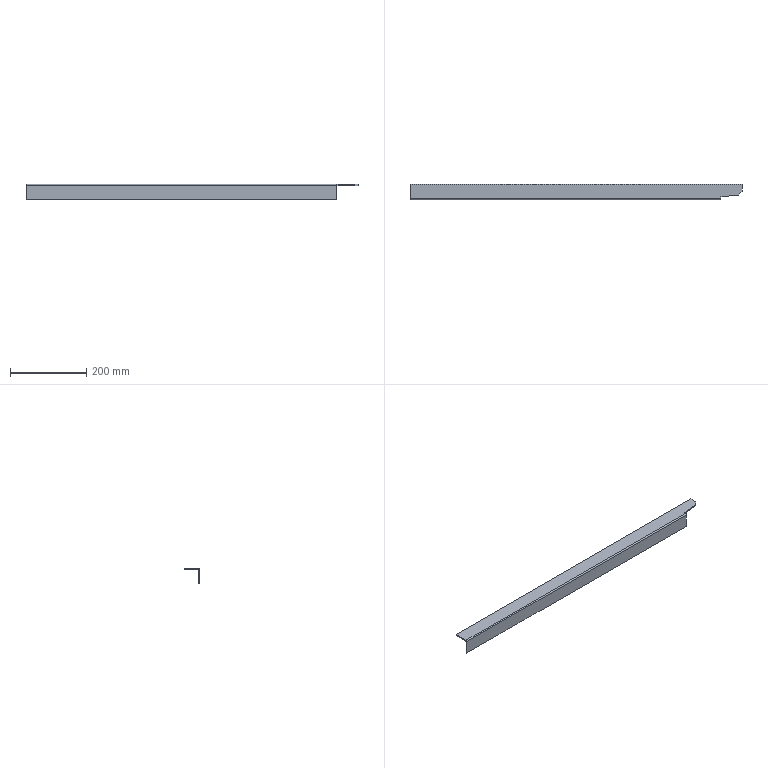Part | SolidWorks | 1 solid | 18 faces | box 873.5 x 40 x 40 mm | volume 192005 mm3 | plane 16 | cylinder 2 | commonest cylinder face diameters 0.2 x1 6.2 x1
STEP:
#1=CARTESIAN_POINT('',(380.25,0.,-40.));
#2=VERTEX_POINT('',#1);
#3=CARTESIAN_POINT('',(380.25,0.,-3.1));
#4=VERTEX_POINT('',#3);
#5=CARTESIAN_POINT('',(380.25,0.,0.));
#6=DIRECTION('',(0.,0.,1.));
#7=VECTOR('',#6,1000.);
#8=LINE('',#5,#7);
#9=EDGE_CURVE('',#2,#4,#8,.T.);
#10=ORIENTED_EDGE('',*,*,#9,.T.);
#11=CARTESIAN_POINT('',(-436.75,0.,-3.1));
#12=VERTEX_POINT('',#11);
#13=CARTESIAN_POINT('',(436.75,0.,-3.1));
#14=DIRECTION('',(-1.,0.,0.));
#15=VECTOR('',#14,1000.);
#16=LINE('',#13,#15);
#17=EDGE_CURVE('',#4,#12,#16,.T.);
#18=ORIENTED_EDGE('',*,*,#17,.T.);
#19=CARTESIAN_POINT('',(-436.75,0.,-40.));
#20=VERTEX_POINT('',#19);
#21=CARTESIAN_POINT('',(-436.75,0.,0.));
#22=DIRECTION('',(0.,0.,-1.));
#23=VECTOR('',#22,1000.);
#24=LINE('',#21,#23);
#25=EDGE_CURVE('',#12,#20,#24,.T.);
#26=ORIENTED_EDGE('',*,*,#25,.T.);
#27=CARTESIAN_POINT('',(436.75,0.,-40.));
#28=DIRECTION('',(-1.,0.,0.));
#29=VECTOR('',#28,1000.);
#30=LINE('',#27,#29);
#31=EDGE_CURVE('',#2,#20,#30,.T.);
#32=ORIENTED_EDGE('',*,*,#31,.F.);
#33=EDGE_LOOP('',(#10,#18,#26,#32));
#34=FACE_OUTER_BOUND('',#33,.T.);
#35=CARTESIAN_POINT('',(436.75,0.,0.));
#36=DIRECTION('',(0.,1.,0.));
#37=DIRECTION('',(0.,0.,1.));
#38=AXIS2_PLACEMENT_3D('',#35,#36,#37);
#39=PLANE('',#38);
#40=ADVANCED_FACE('',(#34),#39,.F.);
#41=CARTESIAN_POINT('',(380.25,3.,-40.));
#42=VERTEX_POINT('',#41);
#43=CARTESIAN_POINT('',(-436.75,3.,-40.));
#44=VERTEX_POINT('',#43);
#45=CARTESIAN_POINT('',(436.75,3.,-40.));
#46=DIRECTION('',(-1.,0.,0.));
#47=VECTOR('',#46,1000.);
#48=LINE('',#45,#47);
#49=EDGE_CURVE('',#42,#44,#48,.T.);
#50=ORIENTED_EDGE('',*,*,#49,.F.);
#51=CARTESIAN_POINT('',(380.25,3.,-40.));
#52=DIRECTION('',(0.,-1.,0.));
#53=VECTOR('',#52,1000.);
#54=LINE('',#51,#53);
#55=EDGE_CURVE('',#42,#2,#54,.T.);
#56=ORIENTED_EDGE('',*,*,#55,.T.);
#57=ORIENTED_EDGE('',*,*,#31,.T.);
#58=CARTESIAN_POINT('',(-436.75,3.,-40.));
#59=DIRECTION('',(0.,-1.,0.));
#60=VECTOR('',#59,1000.);
#61=LINE('',#58,#60);
#62=EDGE_CURVE('',#44,#20,#61,.T.);
#63=ORIENTED_EDGE('',*,*,#62,.F.);
#64=EDGE_LOOP('',(#50,#56,#57,#63));
#65=FACE_OUTER_BOUND('',#64,.T.);
#66=CARTESIAN_POINT('',(436.75,3.,-40.));
#67=DIRECTION('',(0.,0.,-1.));
#68=DIRECTION('',(-1.,0.,0.));
#69=AXIS2_PLACEMENT_3D('',#66,#67,#68);
#70=PLANE('',#69);
#71=ADVANCED_FACE('',(#65),#70,.T.);
#72=CARTESIAN_POINT('',(380.25,3.,-3.1));
#73=VERTEX_POINT('',#72);
#74=CARTESIAN_POINT('',(-436.75,3.,-3.1));
#75=VERTEX_POINT('',#74);
#76=CARTESIAN_POINT('',(436.75,3.,-3.1));
#77=DIRECTION('',(-1.,0.,0.));
#78=VECTOR('',#77,1000.);
#79=LINE('',#76,#78);
#80=EDGE_CURVE('',#73,#75,#79,.T.);
#81=ORIENTED_EDGE('',*,*,#80,.F.);
#82=CARTESIAN_POINT('',(380.25,3.,0.));
#83=DIRECTION('',(0.,0.,1.));
#84=VECTOR('',#83,1000.);
#85=LINE('',#82,#84);
#86=EDGE_CURVE('',#42,#73,#85,.T.);
#87=ORIENTED_EDGE('',*,*,#86,.F.);
#88=ORIENTED_EDGE('',*,*,#49,.T.);
#89=CARTESIAN_POINT('',(-436.75,3.,0.));
#90=DIRECTION('',(0.,0.,-1.));
#91=VECTOR('',#90,1000.);
#92=LINE('',#89,#91);
#93=EDGE_CURVE('',#75,#44,#92,.T.);
#94=ORIENTED_EDGE('',*,*,#93,.F.);
#95=EDGE_LOOP('',(#81,#87,#88,#94));
#96=FACE_OUTER_BOUND('',#95,.T.);
#97=CARTESIAN_POINT('',(436.75,3.,0.));
#98=DIRECTION('',(0.,1.,0.));
#99=DIRECTION('',(0.,0.,1.));
#100=AXIS2_PLACEMENT_3D('',#97,#98,#99);
#101=PLANE('',#100);
#102=ADVANCED_FACE('',(#96),#101,.T.);
#103=CARTESIAN_POINT('',(380.25,3.1,-3.));
#104=VERTEX_POINT('',#103);
#105=CARTESIAN_POINT('',(-436.75,3.1,-3.));
#106=VERTEX_POINT('',#105);
#107=CARTESIAN_POINT('',(436.75,3.1,-3.));
#108=DIRECTION('',(-1.,0.,0.));
#109=VECTOR('',#108,1000.);
#110=LINE('',#107,#109);
#111=EDGE_CURVE('',#104,#106,#110,.T.);
#112=ORIENTED_EDGE('',*,*,#111,.F.);
#113=CARTESIAN_POINT('',(380.25,3.1,-3.1));
#114=DIRECTION('',(-1.,0.,0.));
#115=DIRECTION('',(0.,0.,1.));
#116=AXIS2_PLACEMENT_3D('',#113,#114,#115);
#117=CIRCLE('',#116,0.1);
#118=EDGE_CURVE('',#73,#104,#117,.T.);
#119=ORIENTED_EDGE('',*,*,#118,.F.);
#120=ORIENTED_EDGE('',*,*,#80,.T.);
#121=CARTESIAN_POINT('',(-436.75,3.1,-3.1));
#122=DIRECTION('',(1.,0.,0.));
#123=DIRECTION('',(0.,0.,-1.));
#124=AXIS2_PLACEMENT_3D('',#121,#122,#123);
#125=CIRCLE('',#124,0.1);
#126=EDGE_CURVE('',#106,#75,#125,.T.);
#127=ORIENTED_EDGE('',*,*,#126,.F.);
#128=EDGE_LOOP('',(#112,#119,#120,#127));
#129=FACE_OUTER_BOUND('',#128,.T.);
#130=CARTESIAN_POINT('',(436.75,3.1,-3.1));
#131=DIRECTION('',(-1.,0.,0.));
#132=DIRECTION('',(0.,0.,1.));
#133=AXIS2_PLACEMENT_3D('',#130,#131,#132);
#134=CYLINDRICAL_SURFACE('',#133,0.1);
#135=ADVANCED_FACE('',(#129),#134,.F.);
#136=CARTESIAN_POINT('',(436.75,40.,-3.));
#137=VERTEX_POINT('',#136);
#138=CARTESIAN_POINT('',(436.75,21.973,-3.));
#139=VERTEX_POINT('',#138);
#140=CARTESIAN_POINT('',(436.75,40.,-3.));
#141=DIRECTION('',(0.,-1.,0.));
#142=VECTOR('',#141,1000.);
#143=LINE('',#140,#142);
#144=EDGE_CURVE('',#137,#139,#143,.T.);
#145=ORIENTED_EDGE('',*,*,#144,.T.);
#146=CARTESIAN_POINT('',(427.795,12.028,-3.));
#147=VERTEX_POINT('',#146);
#148=CARTESIAN_POINT('',(427.795,12.028,-3.));
#149=DIRECTION('',(-0.6691,-0.7431,0.));
#150=VECTOR('',#149,1000.);
#151=LINE('',#148,#150);
#152=EDGE_CURVE('',#139,#147,#151,.T.);
#153=ORIENTED_EDGE('',*,*,#152,.T.);
#154=CARTESIAN_POINT('',(384.727,7.501,-3.));
#155=VERTEX_POINT('',#154);
#156=CARTESIAN_POINT('',(384.727,7.501,-3.));
#157=DIRECTION('',(-0.9945,-0.1045,0.));
#158=VECTOR('',#157,1000.);
#159=LINE('',#156,#158);
#160=EDGE_CURVE('',#147,#155,#159,.T.);
#161=ORIENTED_EDGE('',*,*,#160,.T.);
#162=CARTESIAN_POINT('',(380.25,7.501,-3.));
#163=VERTEX_POINT('',#162);
#164=CARTESIAN_POINT('',(436.75,7.501,-3.));
#165=DIRECTION('',(-1.,0.,0.));
#166=VECTOR('',#165,1000.);
#167=LINE('',#164,#166);
#168=EDGE_CURVE('',#155,#163,#167,.T.);
#169=ORIENTED_EDGE('',*,*,#168,.T.);
#170=CARTESIAN_POINT('',(380.25,40.,-3.));
#171=DIRECTION('',(0.,-1.,0.));
#172=VECTOR('',#171,1000.);
#173=LINE('',#170,#172);
#174=EDGE_CURVE('',#163,#104,#173,.T.);
#175=ORIENTED_EDGE('',*,*,#174,.T.);
#176=ORIENTED_EDGE('',*,*,#111,.T.);
#177=CARTESIAN_POINT('',(-436.75,40.,-3.));
#178=VERTEX_POINT('',#177);
#179=CARTESIAN_POINT('',(-436.75,40.,-3.));
#180=DIRECTION('',(0.,-1.,0.));
#181=VECTOR('',#180,1000.);
#182=LINE('',#179,#181);
#183=EDGE_CURVE('',#178,#106,#182,.T.);
#184=ORIENTED_EDGE('',*,*,#183,.F.);
#185=CARTESIAN_POINT('',(436.75,40.,-3.));
#186=DIRECTION('',(-1.,0.,0.));
#187=VECTOR('',#186,1000.);
#188=LINE('',#185,#187);
#189=EDGE_CURVE('',#137,#178,#188,.T.);
#190=ORIENTED_EDGE('',*,*,#189,.F.);
#191=EDGE_LOOP('',(#145,#153,#161,#169,#175,#176,#184,#190));
#192=FACE_OUTER_BOUND('',#191,.T.);
#193=CARTESIAN_POINT('',(436.75,40.,-3.));
#194=DIRECTION('',(0.,0.,-1.));
#195=DIRECTION('',(0.,1.,0.));
#196=AXIS2_PLACEMENT_3D('',#193,#194,#195);
#197=PLANE('',#196);
#198=ADVANCED_FACE('',(#192),#197,.T.);
#199=CARTESIAN_POINT('',(436.75,21.973,0.));
#200=VERTEX_POINT('',#199);
#201=CARTESIAN_POINT('',(427.795,12.028,0.));
#202=VERTEX_POINT('',#201);
#203=CARTESIAN_POINT('',(427.795,12.028,0.));
#204=DIRECTION('',(-0.6691,-0.7431,0.));
#205=VECTOR('',#204,1000.);
#206=LINE('',#203,#205);
#207=EDGE_CURVE('',#200,#202,#206,.T.);
#208=ORIENTED_EDGE('',*,*,#207,.F.);
#209=CARTESIAN_POINT('',(436.75,40.,0.));
#210=VERTEX_POINT('',#209);
#211=CARTESIAN_POINT('',(436.75,40.,0.));
#212=DIRECTION('',(0.,-1.,0.));
#213=VECTOR('',#212,1000.);
#214=LINE('',#211,#213);
#215=EDGE_CURVE('',#210,#200,#214,.T.);
#216=ORIENTED_EDGE('',*,*,#215,.F.);
#217=CARTESIAN_POINT('',(-436.75,40.,0.));
#218=VERTEX_POINT('',#217);
#219=CARTESIAN_POINT('',(436.75,40.,0.));
#220=DIRECTION('',(-1.,0.,0.));
#221=VECTOR('',#220,1000.);
#222=LINE('',#219,#221);
#223=EDGE_CURVE('',#210,#218,#222,.T.);
#224=ORIENTED_EDGE('',*,*,#223,.T.);
#225=CARTESIAN_POINT('',(-436.75,3.1,0.));
#226=VERTEX_POINT('',#225);
#227=CARTESIAN_POINT('',(-436.75,40.,0.));
#228=DIRECTION('',(0.,-1.,0.));
#229=VECTOR('',#228,1000.);
#230=LINE('',#227,#229);
#231=EDGE_CURVE('',#218,#226,#230,.T.);
#232=ORIENTED_EDGE('',*,*,#231,.T.);
#233=CARTESIAN_POINT('',(380.25,3.1,0.));
#234=VERTEX_POINT('',#233);
#235=CARTESIAN_POINT('',(436.75,3.1,0.));
#236=DIRECTION('',(-1.,0.,0.));
#237=VECTOR('',#236,1000.);
#238=LINE('',#235,#237);
#239=EDGE_CURVE('',#234,#226,#238,.T.);
#240=ORIENTED_EDGE('',*,*,#239,.F.);
#241=CARTESIAN_POINT('',(380.25,7.501,0.));
#242=VERTEX_POINT('',#241);
#243=CARTESIAN_POINT('',(380.25,-5.,0.));
#244=DIRECTION('',(0.,-1.,0.));
#245=VECTOR('',#244,1000.);
#246=LINE('',#243,#245);
#247=EDGE_CURVE('',#242,#234,#246,.T.);
#248=ORIENTED_EDGE('',*,*,#247,.F.);
#249=CARTESIAN_POINT('',(384.727,7.501,0.));
#250=VERTEX_POINT('',#249);
#251=CARTESIAN_POINT('',(380.25,7.501,0.));
#252=DIRECTION('',(-1.,0.,0.));
#253=VECTOR('',#252,1000.);
#254=LINE('',#251,#253);
#255=EDGE_CURVE('',#250,#242,#254,.T.);
#256=ORIENTED_EDGE('',*,*,#255,.F.);
#257=CARTESIAN_POINT('',(384.727,7.501,0.));
#258=DIRECTION('',(-0.9945,-0.1045,0.));
#259=VECTOR('',#258,1000.);
#260=LINE('',#257,#259);
#261=EDGE_CURVE('',#202,#250,#260,.T.);
#262=ORIENTED_EDGE('',*,*,#261,.F.);
#263=EDGE_LOOP('',(#208,#216,#224,#232,#240,#248,#256,#262));
#264=FACE_OUTER_BOUND('',#263,.T.);
#265=CARTESIAN_POINT('',(436.75,40.,0.));
#266=DIRECTION('',(0.,0.,-1.));
#267=DIRECTION('',(0.,1.,0.));
#268=AXIS2_PLACEMENT_3D('',#265,#266,#267);
#269=PLANE('',#268);
#270=ADVANCED_FACE('',(#264),#269,.F.);
#271=CARTESIAN_POINT('',(380.25,3.1,-3.1));
#272=DIRECTION('',(-1.,0.,0.));
#273=DIRECTION('',(0.,0.,1.));
#274=AXIS2_PLACEMENT_3D('',#271,#272,#273);
#275=CIRCLE('',#274,3.1);
#276=EDGE_CURVE('',#4,#234,#275,.T.);
#277=ORIENTED_EDGE('',*,*,#276,.T.);
#278=ORIENTED_EDGE('',*,*,#239,.T.);
#279=CARTESIAN_POINT('',(-436.75,3.1,-3.1));
#280=DIRECTION('',(1.,0.,0.));
#281=DIRECTION('',(0.,0.,1.));
#282=AXIS2_PLACEMENT_3D('',#279,#280,#281);
#283=CIRCLE('',#282,3.1);
#284=EDGE_CURVE('',#226,#12,#283,.T.);
#285=ORIENTED_EDGE('',*,*,#284,.T.);
#286=ORIENTED_EDGE('',*,*,#17,.F.);
#287=EDGE_LOOP('',(#277,#278,#285,#286));
#288=FACE_OUTER_BOUND('',#287,.T.);
#289=CARTESIAN_POINT('',(436.75,3.1,-3.1));
#290=DIRECTION('',(-1.,0.,0.));
#291=DIRECTION('',(0.,0.,1.));
#292=AXIS2_PLACEMENT_3D('',#289,#290,#291);
#293=CYLINDRICAL_SURFACE('',#292,3.1);
#294=ADVANCED_FACE('',(#288),#293,.T.);
#295=ORIENTED_EDGE('',*,*,#215,.T.);
#296=CARTESIAN_POINT('',(436.75,21.973,0.));
#297=DIRECTION('',(0.,0.,-1.));
#298=VECTOR('',#297,1000.);
#299=LINE('',#296,#298);
#300=EDGE_CURVE('',#200,#139,#299,.T.);
#301=ORIENTED_EDGE('',*,*,#300,.T.);
#302=ORIENTED_EDGE('',*,*,#144,.F.);
#303=CARTESIAN_POINT('',(436.75,40.,0.));
#304=DIRECTION('',(0.,0.,-1.));
#305=VECTOR('',#304,1000.);
#306=LINE('',#303,#305);
#307=EDGE_CURVE('',#210,#137,#306,.T.);
#308=ORIENTED_EDGE('',*,*,#307,.F.);
#309=EDGE_LOOP('',(#295,#301,#302,#308));
#310=FACE_OUTER_BOUND('',#309,.T.);
#311=CARTESIAN_POINT('',(436.75,3.,-3.1));
#312=DIRECTION('',(1.,0.,0.));
#313=DIRECTION('',(0.,0.,-1.));
#314=AXIS2_PLACEMENT_3D('',#311,#312,#313);
#315=PLANE('',#314);
#316=ADVANCED_FACE('',(#310),#315,.T.);
#317=CARTESIAN_POINT('',(-436.75,0.,-3.1));
#318=DIRECTION('',(0.,1.,0.));
#319=VECTOR('',#318,1000.);
#320=LINE('',#317,#319);
#321=EDGE_CURVE('',#12,#75,#320,.T.);
#322=ORIENTED_EDGE('',*,*,#321,.F.);
#323=ORIENTED_EDGE('',*,*,#284,.F.);
#324=CARTESIAN_POINT('',(-436.75,3.1,-3.));
#325=DIRECTION('',(0.,0.,1.));
#326=VECTOR('',#325,1000.);
#327=LINE('',#324,#326);
#328=EDGE_CURVE('',#106,#226,#327,.T.);
#329=ORIENTED_EDGE('',*,*,#328,.F.);
#330=ORIENTED_EDGE('',*,*,#126,.T.);
#331=EDGE_LOOP('',(#322,#323,#329,#330));
#332=FACE_OUTER_BOUND('',#331,.T.);
#333=CARTESIAN_POINT('',(-436.75,0.,-3.1));
#334=DIRECTION('',(-1.,0.,0.));
#335=DIRECTION('',(0.,0.,1.));
#336=AXIS2_PLACEMENT_3D('',#333,#334,#335);
#337=PLANE('',#336);
#338=ADVANCED_FACE('',(#332),#337,.T.);
#339=ORIENTED_EDGE('',*,*,#25,.F.);
#340=ORIENTED_EDGE('',*,*,#321,.T.);
#341=ORIENTED_EDGE('',*,*,#93,.T.);
#342=ORIENTED_EDGE('',*,*,#62,.T.);
#343=EDGE_LOOP('',(#339,#340,#341,#342));
#344=FACE_OUTER_BOUND('',#343,.T.);
#345=CARTESIAN_POINT('',(-436.75,3.1,-3.));
#346=DIRECTION('',(-1.,0.,0.));
#347=DIRECTION('',(0.,0.,1.));
#348=AXIS2_PLACEMENT_3D('',#345,#346,#347);
#349=PLANE('',#348);
#350=ADVANCED_FACE('',(#344),#349,.T.);
#351=CARTESIAN_POINT('',(-436.75,40.,0.));
#352=DIRECTION('',(0.,0.,-1.));
#353=VECTOR('',#352,1000.);
#354=LINE('',#351,#353);
#355=EDGE_CURVE('',#218,#178,#354,.T.);
#356=ORIENTED_EDGE('',*,*,#355,.F.);
#357=ORIENTED_EDGE('',*,*,#223,.F.);
#358=ORIENTED_EDGE('',*,*,#307,.T.);
#359=ORIENTED_EDGE('',*,*,#189,.T.);
#360=EDGE_LOOP('',(#356,#357,#358,#359));
#361=FACE_OUTER_BOUND('',#360,.T.);
#362=CARTESIAN_POINT('',(436.75,40.,0.));
#363=DIRECTION('',(0.,1.,0.));
#364=DIRECTION('',(0.,0.,1.));
#365=AXIS2_PLACEMENT_3D('',#362,#363,#364);
#366=PLANE('',#365);
#367=ADVANCED_FACE('',(#361),#366,.T.);
#368=ORIENTED_EDGE('',*,*,#183,.T.);
#369=ORIENTED_EDGE('',*,*,#328,.T.);
#370=ORIENTED_EDGE('',*,*,#231,.F.);
#371=ORIENTED_EDGE('',*,*,#355,.T.);
#372=EDGE_LOOP('',(#368,#369,#370,#371));
#373=FACE_OUTER_BOUND('',#372,.T.);
#374=CARTESIAN_POINT('',(-436.75,3.1,-3.1));
#375=DIRECTION('',(1.,0.,0.));
#376=DIRECTION('',(0.,0.,-1.));
#377=AXIS2_PLACEMENT_3D('',#374,#375,#376);
#378=PLANE('',#377);
#379=ADVANCED_FACE('',(#373),#378,.F.);
#380=ORIENTED_EDGE('',*,*,#86,.T.);
#381=CARTESIAN_POINT('',(380.25,3.,-3.1));
#382=DIRECTION('',(0.,-1.,0.));
#383=VECTOR('',#382,1000.);
#384=LINE('',#381,#383);
#385=EDGE_CURVE('',#73,#4,#384,.T.);
#386=ORIENTED_EDGE('',*,*,#385,.T.);
#387=ORIENTED_EDGE('',*,*,#9,.F.);
#388=ORIENTED_EDGE('',*,*,#55,.F.);
#389=EDGE_LOOP('',(#380,#386,#387,#388));
#390=FACE_OUTER_BOUND('',#389,.T.);
#391=CARTESIAN_POINT('',(380.25,3.,0.));
#392=DIRECTION('',(-1.,0.,0.));
#393=DIRECTION('',(0.,0.,1.));
#394=AXIS2_PLACEMENT_3D('',#391,#392,#393);
#395=PLANE('',#394);
#396=ADVANCED_FACE('',(#390),#395,.F.);
#397=ORIENTED_EDGE('',*,*,#300,.F.);
#398=ORIENTED_EDGE('',*,*,#207,.T.);
#399=CARTESIAN_POINT('',(427.795,12.028,0.));
#400=DIRECTION('',(0.,0.,-1.));
#401=VECTOR('',#400,1000.);
#402=LINE('',#399,#401);
#403=EDGE_CURVE('',#202,#147,#402,.T.);
#404=ORIENTED_EDGE('',*,*,#403,.T.);
#405=ORIENTED_EDGE('',*,*,#152,.F.);
#406=EDGE_LOOP('',(#397,#398,#404,#405));
#407=FACE_OUTER_BOUND('',#406,.T.);
#408=CARTESIAN_POINT('',(427.795,12.028,0.));
#409=DIRECTION('',(0.7431,-0.6691,0.));
#410=DIRECTION('',(-0.6691,-0.7431,0.));
#411=AXIS2_PLACEMENT_3D('',#408,#409,#410);
#412=PLANE('',#411);
#413=ADVANCED_FACE('',(#407),#412,.T.);
#414=ORIENTED_EDGE('',*,*,#403,.F.);
#415=ORIENTED_EDGE('',*,*,#261,.T.);
#416=CARTESIAN_POINT('',(384.727,7.501,0.));
#417=DIRECTION('',(0.,0.,-1.));
#418=VECTOR('',#417,1000.);
#419=LINE('',#416,#418);
#420=EDGE_CURVE('',#250,#155,#419,.T.);
#421=ORIENTED_EDGE('',*,*,#420,.T.);
#422=ORIENTED_EDGE('',*,*,#160,.F.);
#423=EDGE_LOOP('',(#414,#415,#421,#422));
#424=FACE_OUTER_BOUND('',#423,.T.);
#425=CARTESIAN_POINT('',(384.727,7.501,0.));
#426=DIRECTION('',(0.1045,-0.9945,0.));
#427=DIRECTION('',(-0.9945,-0.1045,0.));
#428=AXIS2_PLACEMENT_3D('',#425,#426,#427);
#429=PLANE('',#428);
#430=ADVANCED_FACE('',(#424),#429,.T.);
#431=ORIENTED_EDGE('',*,*,#420,.F.);
#432=ORIENTED_EDGE('',*,*,#255,.T.);
#433=CARTESIAN_POINT('',(380.25,7.501,0.));
#434=DIRECTION('',(0.,0.,-1.));
#435=VECTOR('',#434,1000.);
#436=LINE('',#433,#435);
#437=EDGE_CURVE('',#242,#163,#436,.T.);
#438=ORIENTED_EDGE('',*,*,#437,.T.);
#439=ORIENTED_EDGE('',*,*,#168,.F.);
#440=EDGE_LOOP('',(#431,#432,#438,#439));
#441=FACE_OUTER_BOUND('',#440,.T.);
#442=CARTESIAN_POINT('',(380.25,7.501,0.));
#443=DIRECTION('',(0.,-1.,0.));
#444=DIRECTION('',(-1.,0.,0.));
#445=AXIS2_PLACEMENT_3D('',#442,#443,#444);
#446=PLANE('',#445);
#447=ADVANCED_FACE('',(#441),#446,.T.);
#448=ORIENTED_EDGE('',*,*,#437,.F.);
#449=ORIENTED_EDGE('',*,*,#247,.T.);
#450=CARTESIAN_POINT('',(380.25,3.1,0.));
#451=DIRECTION('',(0.,0.,-1.));
#452=VECTOR('',#451,1000.);
#453=LINE('',#450,#452);
#454=EDGE_CURVE('',#234,#104,#453,.T.);
#455=ORIENTED_EDGE('',*,*,#454,.T.);
#456=ORIENTED_EDGE('',*,*,#174,.F.);
#457=EDGE_LOOP('',(#448,#449,#455,#456));
#458=FACE_OUTER_BOUND('',#457,.T.);
#459=CARTESIAN_POINT('',(380.25,-5.,0.));
#460=DIRECTION('',(1.,0.,0.));
#461=DIRECTION('',(0.,-1.,0.));
#462=AXIS2_PLACEMENT_3D('',#459,#460,#461);
#463=PLANE('',#462);
#464=ADVANCED_FACE('',(#458),#463,.T.);
#465=ORIENTED_EDGE('',*,*,#454,.F.);
#466=ORIENTED_EDGE('',*,*,#276,.F.);
#467=ORIENTED_EDGE('',*,*,#385,.F.);
#468=ORIENTED_EDGE('',*,*,#118,.T.);
#469=EDGE_LOOP('',(#465,#466,#467,#468));
#470=FACE_OUTER_BOUND('',#469,.T.);
#471=CARTESIAN_POINT('',(380.25,3.1,-3.1));
#472=DIRECTION('',(1.,0.,0.));
#473=DIRECTION('',(0.,0.,-1.));
#474=AXIS2_PLACEMENT_3D('',#471,#472,#473);
#475=PLANE('',#474);
#476=ADVANCED_FACE('',(#470),#475,.T.);
#477=CLOSED_SHELL('',(#40,#71,#102,#135,#198,#270,#294,#316,#338,#350,#367,#379,#396,#413,#430,#447,#464,#476));
#478=MANIFOLD_SOLID_BREP('',#477);
#479=CARTESIAN_POINT('',(0.,0.,0.));
#480=DIRECTION('',(0.,0.,1.));
#481=DIRECTION('',(1.,0.,0.));
#482=AXIS2_PLACEMENT_3D('',#479,#480,#481);
#483=(LENGTH_UNIT()NAMED_UNIT(*)SI_UNIT(.MILLI.,.METRE.));
#484=UNCERTAINTY_MEASURE_WITH_UNIT(LENGTH_MEASURE(0.00001),#483,'','');
#485=(NAMED_UNIT(*)PLANE_ANGLE_UNIT()SI_UNIT($,.RADIAN.));
#486=(NAMED_UNIT(*)SI_UNIT($,.STERADIAN.)SOLID_ANGLE_UNIT());
#487=(GEOMETRIC_REPRESENTATION_CONTEXT(3)GLOBAL_UNCERTAINTY_ASSIGNED_CONTEXT((#484))GLOBAL_UNIT_ASSIGNED_CONTEXT((#483,#485,#486))REPRESENTATION_CONTEXT('',''));
#488=ADVANCED_BREP_SHAPE_REPRESENTATION('',(#478,#482),#487);